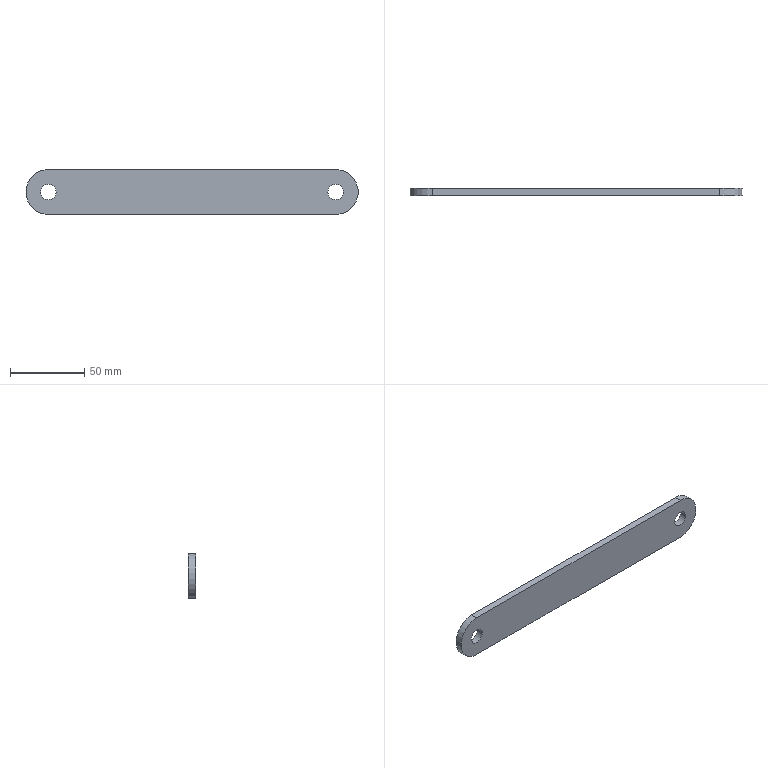Part | NX | features BREP 1 | 1 solid | 10 faces | box 223.202 x 4.763 x 30.163 mm | volume 30322 mm3 | cylinder 6 | plane 4 | commonest cylinder face diameters 10.414 x4 30.163 x2
STEP:
#1=CARTESIAN_POINT('',(-96.52,0.,15.081));
#2=VERTEX_POINT('',#1);
#3=CARTESIAN_POINT('',(96.52,0.,15.081));
#4=VERTEX_POINT('',#3);
#5=CARTESIAN_POINT('',(-96.52,0.,15.081));
#6=DIRECTION('',(1.,0.,0.));
#7=VECTOR('',#6,1000.);
#8=LINE('',#5,#7);
#9=EDGE_CURVE('',#2,#4,#8,.T.);
#10=ORIENTED_EDGE('',*,*,#9,.T.);
#11=CARTESIAN_POINT('',(96.52,0.,-15.081));
#12=VERTEX_POINT('',#11);
#13=CARTESIAN_POINT('',(96.52,0.,0.));
#14=DIRECTION('',(0.,1.,0.));
#15=DIRECTION('',(0.,0.,1.));
#16=AXIS2_PLACEMENT_3D('',#13,#14,#15);
#17=CIRCLE('',#16,15.081);
#18=EDGE_CURVE('',#4,#12,#17,.T.);
#19=ORIENTED_EDGE('',*,*,#18,.T.);
#20=CARTESIAN_POINT('',(-96.52,0.,-15.081));
#21=VERTEX_POINT('',#20);
#22=CARTESIAN_POINT('',(96.52,0.,-15.081));
#23=DIRECTION('',(-1.,0.,0.));
#24=VECTOR('',#23,1000.);
#25=LINE('',#22,#24);
#26=EDGE_CURVE('',#12,#21,#25,.T.);
#27=ORIENTED_EDGE('',*,*,#26,.T.);
#28=CARTESIAN_POINT('',(-96.52,0.,0.));
#29=DIRECTION('',(0.,1.,0.));
#30=DIRECTION('',(0.,0.,-1.));
#31=AXIS2_PLACEMENT_3D('',#28,#29,#30);
#32=CIRCLE('',#31,15.081);
#33=EDGE_CURVE('',#21,#2,#32,.T.);
#34=ORIENTED_EDGE('',*,*,#33,.T.);
#35=EDGE_LOOP('',(#10,#19,#27,#34));
#36=FACE_BOUND('',#35,.T.);
#37=CARTESIAN_POINT('',(91.313,0.,0.));
#38=VERTEX_POINT('',#37);
#39=CARTESIAN_POINT('',(101.727,0.,0.));
#40=VERTEX_POINT('',#39);
#41=CARTESIAN_POINT('',(96.52,0.,0.));
#42=DIRECTION('',(0.,-1.,0.));
#43=DIRECTION('',(-1.,0.,0.));
#44=AXIS2_PLACEMENT_3D('',#41,#42,#43);
#45=CIRCLE('',#44,5.207);
#46=EDGE_CURVE('',#38,#40,#45,.T.);
#47=ORIENTED_EDGE('',*,*,#46,.T.);
#48=CARTESIAN_POINT('',(96.52,0.,0.));
#49=DIRECTION('',(0.,-1.,0.));
#50=DIRECTION('',(1.,0.,0.));
#51=AXIS2_PLACEMENT_3D('',#48,#49,#50);
#52=CIRCLE('',#51,5.207);
#53=EDGE_CURVE('',#40,#38,#52,.T.);
#54=ORIENTED_EDGE('',*,*,#53,.T.);
#55=EDGE_LOOP('',(#47,#54));
#56=FACE_BOUND('',#55,.T.);
#57=CARTESIAN_POINT('',(-101.727,0.,0.));
#58=VERTEX_POINT('',#57);
#59=CARTESIAN_POINT('',(-91.313,0.,0.));
#60=VERTEX_POINT('',#59);
#61=CARTESIAN_POINT('',(-96.52,0.,0.));
#62=DIRECTION('',(0.,-1.,0.));
#63=DIRECTION('',(-1.,0.,0.));
#64=AXIS2_PLACEMENT_3D('',#61,#62,#63);
#65=CIRCLE('',#64,5.207);
#66=EDGE_CURVE('',#58,#60,#65,.T.);
#67=ORIENTED_EDGE('',*,*,#66,.T.);
#68=CARTESIAN_POINT('',(-96.52,0.,0.));
#69=DIRECTION('',(0.,-1.,0.));
#70=DIRECTION('',(1.,0.,0.));
#71=AXIS2_PLACEMENT_3D('',#68,#69,#70);
#72=CIRCLE('',#71,5.207);
#73=EDGE_CURVE('',#60,#58,#72,.T.);
#74=ORIENTED_EDGE('',*,*,#73,.T.);
#75=EDGE_LOOP('',(#67,#74));
#76=FACE_BOUND('',#75,.T.);
#77=CARTESIAN_POINT('',(0.,0.,0.));
#78=DIRECTION('',(0.,1.,0.));
#79=DIRECTION('',(1.,0.,0.));
#80=AXIS2_PLACEMENT_3D('',#77,#78,#79);
#81=PLANE('',#80);
#82=ADVANCED_FACE('',(#36,#56,#76),#81,.T.);
#83=CARTESIAN_POINT('',(-96.52,-4.763,-15.081));
#84=VERTEX_POINT('',#83);
#85=CARTESIAN_POINT('',(-96.52,0.,-15.081));
#86=DIRECTION('',(0.,-1.,0.));
#87=VECTOR('',#86,1000.);
#88=LINE('',#85,#87);
#89=EDGE_CURVE('',#21,#84,#88,.T.);
#90=ORIENTED_EDGE('',*,*,#89,.T.);
#91=CARTESIAN_POINT('',(-96.52,-4.763,15.081));
#92=VERTEX_POINT('',#91);
#93=CARTESIAN_POINT('',(-96.52,-4.763,0.));
#94=DIRECTION('',(0.,1.,0.));
#95=DIRECTION('',(0.,0.,-1.));
#96=AXIS2_PLACEMENT_3D('',#93,#94,#95);
#97=CIRCLE('',#96,15.081);
#98=EDGE_CURVE('',#84,#92,#97,.T.);
#99=ORIENTED_EDGE('',*,*,#98,.T.);
#100=CARTESIAN_POINT('',(-96.52,0.,15.081));
#101=DIRECTION('',(0.,-1.,0.));
#102=VECTOR('',#101,1000.);
#103=LINE('',#100,#102);
#104=EDGE_CURVE('',#2,#92,#103,.T.);
#105=ORIENTED_EDGE('',*,*,#104,.F.);
#106=ORIENTED_EDGE('',*,*,#33,.F.);
#107=EDGE_LOOP('',(#90,#99,#105,#106));
#108=FACE_BOUND('',#107,.T.);
#109=CARTESIAN_POINT('',(-96.52,-2.381,0.));
#110=DIRECTION('',(0.,1.,0.));
#111=DIRECTION('',(0.,0.,-1.));
#112=AXIS2_PLACEMENT_3D('',#109,#110,#111);
#113=CYLINDRICAL_SURFACE('',#112,15.081);
#114=ADVANCED_FACE('',(#108),#113,.T.);
#115=ORIENTED_EDGE('',*,*,#104,.T.);
#116=CARTESIAN_POINT('',(96.52,-4.763,15.081));
#117=VERTEX_POINT('',#116);
#118=CARTESIAN_POINT('',(-96.52,-4.763,15.081));
#119=DIRECTION('',(1.,0.,0.));
#120=VECTOR('',#119,1000.);
#121=LINE('',#118,#120);
#122=EDGE_CURVE('',#92,#117,#121,.T.);
#123=ORIENTED_EDGE('',*,*,#122,.T.);
#124=CARTESIAN_POINT('',(96.52,0.,15.081));
#125=DIRECTION('',(0.,-1.,0.));
#126=VECTOR('',#125,1000.);
#127=LINE('',#124,#126);
#128=EDGE_CURVE('',#4,#117,#127,.T.);
#129=ORIENTED_EDGE('',*,*,#128,.F.);
#130=ORIENTED_EDGE('',*,*,#9,.F.);
#131=EDGE_LOOP('',(#115,#123,#129,#130));
#132=FACE_BOUND('',#131,.T.);
#133=CARTESIAN_POINT('',(0.,-2.381,15.081));
#134=DIRECTION('',(0.,0.,1.));
#135=DIRECTION('',(1.,0.,0.));
#136=AXIS2_PLACEMENT_3D('',#133,#134,#135);
#137=PLANE('',#136);
#138=ADVANCED_FACE('',(#132),#137,.T.);
#139=ORIENTED_EDGE('',*,*,#128,.T.);
#140=CARTESIAN_POINT('',(96.52,-4.763,-15.081));
#141=VERTEX_POINT('',#140);
#142=CARTESIAN_POINT('',(96.52,-4.763,0.));
#143=DIRECTION('',(0.,1.,0.));
#144=DIRECTION('',(0.,0.,1.));
#145=AXIS2_PLACEMENT_3D('',#142,#143,#144);
#146=CIRCLE('',#145,15.081);
#147=EDGE_CURVE('',#117,#141,#146,.T.);
#148=ORIENTED_EDGE('',*,*,#147,.T.);
#149=CARTESIAN_POINT('',(96.52,0.,-15.081));
#150=DIRECTION('',(0.,-1.,0.));
#151=VECTOR('',#150,1000.);
#152=LINE('',#149,#151);
#153=EDGE_CURVE('',#12,#141,#152,.T.);
#154=ORIENTED_EDGE('',*,*,#153,.F.);
#155=ORIENTED_EDGE('',*,*,#18,.F.);
#156=EDGE_LOOP('',(#139,#148,#154,#155));
#157=FACE_BOUND('',#156,.T.);
#158=CARTESIAN_POINT('',(96.52,-2.381,0.));
#159=DIRECTION('',(0.,1.,0.));
#160=DIRECTION('',(0.,0.,1.));
#161=AXIS2_PLACEMENT_3D('',#158,#159,#160);
#162=CYLINDRICAL_SURFACE('',#161,15.081);
#163=ADVANCED_FACE('',(#157),#162,.T.);
#164=ORIENTED_EDGE('',*,*,#153,.T.);
#165=CARTESIAN_POINT('',(96.52,-4.763,-15.081));
#166=DIRECTION('',(-1.,0.,0.));
#167=VECTOR('',#166,1000.);
#168=LINE('',#165,#167);
#169=EDGE_CURVE('',#141,#84,#168,.T.);
#170=ORIENTED_EDGE('',*,*,#169,.T.);
#171=ORIENTED_EDGE('',*,*,#89,.F.);
#172=ORIENTED_EDGE('',*,*,#26,.F.);
#173=EDGE_LOOP('',(#164,#170,#171,#172));
#174=FACE_BOUND('',#173,.T.);
#175=CARTESIAN_POINT('',(0.,-2.381,-15.081));
#176=DIRECTION('',(0.,0.,-1.));
#177=DIRECTION('',(0.,-1.,0.));
#178=AXIS2_PLACEMENT_3D('',#175,#176,#177);
#179=PLANE('',#178);
#180=ADVANCED_FACE('',(#174),#179,.T.);
#181=ORIENTED_EDGE('',*,*,#169,.F.);
#182=ORIENTED_EDGE('',*,*,#147,.F.);
#183=ORIENTED_EDGE('',*,*,#122,.F.);
#184=ORIENTED_EDGE('',*,*,#98,.F.);
#185=EDGE_LOOP('',(#181,#182,#183,#184));
#186=FACE_BOUND('',#185,.T.);
#187=CARTESIAN_POINT('',(91.313,-4.763,0.));
#188=VERTEX_POINT('',#187);
#189=CARTESIAN_POINT('',(101.727,-4.763,0.));
#190=VERTEX_POINT('',#189);
#191=CARTESIAN_POINT('',(96.52,-4.763,0.));
#192=DIRECTION('',(0.,-1.,0.));
#193=DIRECTION('',(-1.,0.,0.));
#194=AXIS2_PLACEMENT_3D('',#191,#192,#193);
#195=CIRCLE('',#194,5.207);
#196=EDGE_CURVE('',#188,#190,#195,.T.);
#197=ORIENTED_EDGE('',*,*,#196,.F.);
#198=CARTESIAN_POINT('',(96.52,-4.763,0.));
#199=DIRECTION('',(0.,-1.,0.));
#200=DIRECTION('',(1.,0.,0.));
#201=AXIS2_PLACEMENT_3D('',#198,#199,#200);
#202=CIRCLE('',#201,5.207);
#203=EDGE_CURVE('',#190,#188,#202,.T.);
#204=ORIENTED_EDGE('',*,*,#203,.F.);
#205=EDGE_LOOP('',(#197,#204));
#206=FACE_BOUND('',#205,.T.);
#207=CARTESIAN_POINT('',(-101.727,-4.763,0.));
#208=VERTEX_POINT('',#207);
#209=CARTESIAN_POINT('',(-91.313,-4.763,0.));
#210=VERTEX_POINT('',#209);
#211=CARTESIAN_POINT('',(-96.52,-4.763,0.));
#212=DIRECTION('',(0.,-1.,0.));
#213=DIRECTION('',(-1.,0.,0.));
#214=AXIS2_PLACEMENT_3D('',#211,#212,#213);
#215=CIRCLE('',#214,5.207);
#216=EDGE_CURVE('',#208,#210,#215,.T.);
#217=ORIENTED_EDGE('',*,*,#216,.F.);
#218=CARTESIAN_POINT('',(-96.52,-4.763,0.));
#219=DIRECTION('',(0.,-1.,0.));
#220=DIRECTION('',(1.,0.,0.));
#221=AXIS2_PLACEMENT_3D('',#218,#219,#220);
#222=CIRCLE('',#221,5.207);
#223=EDGE_CURVE('',#210,#208,#222,.T.);
#224=ORIENTED_EDGE('',*,*,#223,.F.);
#225=EDGE_LOOP('',(#217,#224));
#226=FACE_BOUND('',#225,.T.);
#227=CARTESIAN_POINT('',(0.,-4.763,0.));
#228=DIRECTION('',(0.,1.,0.));
#229=DIRECTION('',(1.,0.,0.));
#230=AXIS2_PLACEMENT_3D('',#227,#228,#229);
#231=PLANE('',#230);
#232=ADVANCED_FACE('',(#186,#206,#226),#231,.F.);
#233=CARTESIAN_POINT('',(101.727,0.,0.));
#234=DIRECTION('',(0.,-1.,0.));
#235=VECTOR('',#234,1000.);
#236=LINE('',#233,#235);
#237=EDGE_CURVE('',#190,#40,#236,.F.);
#238=ORIENTED_EDGE('',*,*,#237,.F.);
#239=ORIENTED_EDGE('',*,*,#203,.T.);
#240=CARTESIAN_POINT('',(91.313,0.,0.));
#241=DIRECTION('',(0.,-1.,0.));
#242=VECTOR('',#241,1000.);
#243=LINE('',#240,#242);
#244=EDGE_CURVE('',#188,#38,#243,.F.);
#245=ORIENTED_EDGE('',*,*,#244,.T.);
#246=ORIENTED_EDGE('',*,*,#53,.F.);
#247=EDGE_LOOP('',(#238,#239,#245,#246));
#248=FACE_BOUND('',#247,.T.);
#249=CARTESIAN_POINT('',(96.52,0.,0.));
#250=DIRECTION('',(0.,-1.,0.));
#251=DIRECTION('',(1.,0.,0.));
#252=AXIS2_PLACEMENT_3D('',#249,#250,#251);
#253=CYLINDRICAL_SURFACE('',#252,5.207);
#254=ADVANCED_FACE('',(#248),#253,.F.);
#255=ORIENTED_EDGE('',*,*,#244,.F.);
#256=ORIENTED_EDGE('',*,*,#196,.T.);
#257=ORIENTED_EDGE('',*,*,#237,.T.);
#258=ORIENTED_EDGE('',*,*,#46,.F.);
#259=EDGE_LOOP('',(#255,#256,#257,#258));
#260=FACE_BOUND('',#259,.T.);
#261=CARTESIAN_POINT('',(96.52,0.,0.));
#262=DIRECTION('',(0.,-1.,0.));
#263=DIRECTION('',(1.,0.,0.));
#264=AXIS2_PLACEMENT_3D('',#261,#262,#263);
#265=CYLINDRICAL_SURFACE('',#264,5.207);
#266=ADVANCED_FACE('',(#260),#265,.F.);
#267=CARTESIAN_POINT('',(-91.313,0.,0.));
#268=DIRECTION('',(0.,-1.,0.));
#269=VECTOR('',#268,1000.);
#270=LINE('',#267,#269);
#271=EDGE_CURVE('',#210,#60,#270,.F.);
#272=ORIENTED_EDGE('',*,*,#271,.F.);
#273=ORIENTED_EDGE('',*,*,#223,.T.);
#274=CARTESIAN_POINT('',(-101.727,0.,0.));
#275=DIRECTION('',(0.,-1.,0.));
#276=VECTOR('',#275,1000.);
#277=LINE('',#274,#276);
#278=EDGE_CURVE('',#208,#58,#277,.F.);
#279=ORIENTED_EDGE('',*,*,#278,.T.);
#280=ORIENTED_EDGE('',*,*,#73,.F.);
#281=EDGE_LOOP('',(#272,#273,#279,#280));
#282=FACE_BOUND('',#281,.T.);
#283=CARTESIAN_POINT('',(-96.52,0.,0.));
#284=DIRECTION('',(0.,-1.,0.));
#285=DIRECTION('',(1.,0.,0.));
#286=AXIS2_PLACEMENT_3D('',#283,#284,#285);
#287=CYLINDRICAL_SURFACE('',#286,5.207);
#288=ADVANCED_FACE('',(#282),#287,.F.);
#289=ORIENTED_EDGE('',*,*,#278,.F.);
#290=ORIENTED_EDGE('',*,*,#216,.T.);
#291=ORIENTED_EDGE('',*,*,#271,.T.);
#292=ORIENTED_EDGE('',*,*,#66,.F.);
#293=EDGE_LOOP('',(#289,#290,#291,#292));
#294=FACE_BOUND('',#293,.T.);
#295=CARTESIAN_POINT('',(-96.52,0.,0.));
#296=DIRECTION('',(0.,-1.,0.));
#297=DIRECTION('',(1.,0.,0.));
#298=AXIS2_PLACEMENT_3D('',#295,#296,#297);
#299=CYLINDRICAL_SURFACE('',#298,5.207);
#300=ADVANCED_FACE('',(#294),#299,.F.);
#301=CLOSED_SHELL('',(#82,#114,#138,#163,#180,#232,#254,#266,#288,#300));
#302=MANIFOLD_SOLID_BREP('',#301);
#303=(LENGTH_UNIT()NAMED_UNIT(*)SI_UNIT(.MILLI.,.METRE.));
#304=UNCERTAINTY_MEASURE_WITH_UNIT(LENGTH_MEASURE(0.00001),#303,'','');
#305=(NAMED_UNIT(*)PLANE_ANGLE_UNIT()SI_UNIT($,.RADIAN.));
#306=(NAMED_UNIT(*)SI_UNIT($,.STERADIAN.)SOLID_ANGLE_UNIT());
#307=(GEOMETRIC_REPRESENTATION_CONTEXT(3)GLOBAL_UNCERTAINTY_ASSIGNED_CONTEXT((#304))GLOBAL_UNIT_ASSIGNED_CONTEXT((#303,#305,#306))REPRESENTATION_CONTEXT('',''));
#308=ADVANCED_BREP_SHAPE_REPRESENTATION('',(#302),#307);